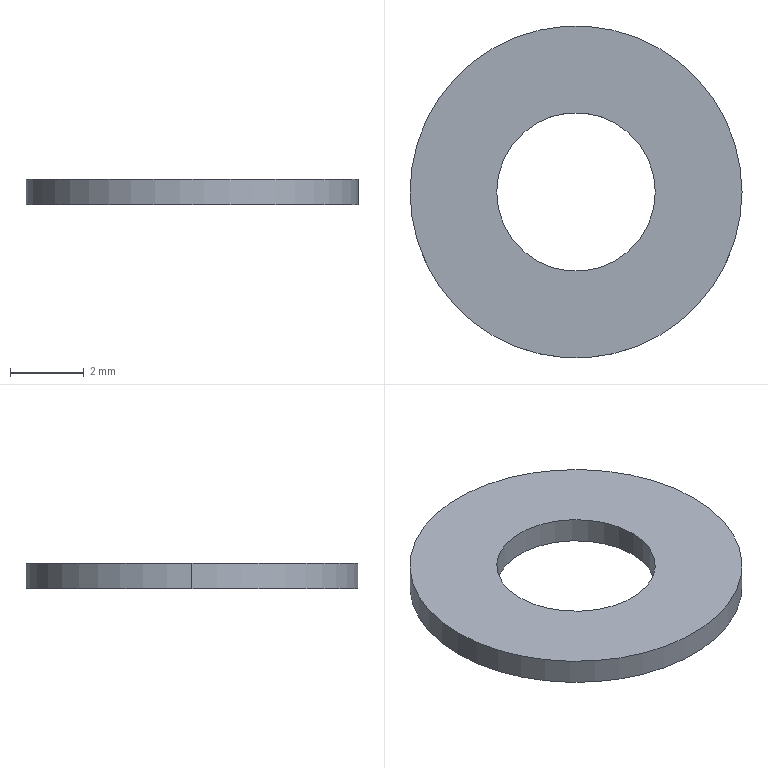Part | SolidWorks | features Extrusion 1, RefAxis 1 | 1 solid | 6 faces | box 9 x 9 x 0.7 mm | volume 34.367 mm3 | cylinder 4 | plane 2 | commonest cylinder face diameters 4.3 x2 9 x2
STEP:
#1=CARTESIAN_POINT('',(-2.15,0.,0.7));
#2=VERTEX_POINT('',#1);
#3=CARTESIAN_POINT('',(2.15,0.,0.7));
#4=VERTEX_POINT('',#3);
#5=CARTESIAN_POINT('',(0.,0.,0.7));
#6=DIRECTION('',(0.,0.,1.));
#7=DIRECTION('',(1.,0.,0.));
#8=AXIS2_PLACEMENT_3D('',#5,#6,#7);
#9=CIRCLE('',#8,2.15);
#10=EDGE_CURVE('',#2,#4,#9,.T.);
#11=ORIENTED_EDGE('',*,*,#10,.T.);
#12=CARTESIAN_POINT('',(2.15,0.,0.));
#13=VERTEX_POINT('',#12);
#14=CARTESIAN_POINT('',(2.15,0.,0.7));
#15=DIRECTION('',(0.,0.,-1.));
#16=VECTOR('',#15,1000.);
#17=LINE('',#14,#16);
#18=EDGE_CURVE('',#4,#13,#17,.T.);
#19=ORIENTED_EDGE('',*,*,#18,.T.);
#20=CARTESIAN_POINT('',(-2.15,0.,0.));
#21=VERTEX_POINT('',#20);
#22=CARTESIAN_POINT('',(0.,0.,0.));
#23=DIRECTION('',(0.,0.,1.));
#24=DIRECTION('',(1.,0.,0.));
#25=AXIS2_PLACEMENT_3D('',#22,#23,#24);
#26=CIRCLE('',#25,2.15);
#27=EDGE_CURVE('',#21,#13,#26,.T.);
#28=ORIENTED_EDGE('',*,*,#27,.F.);
#29=CARTESIAN_POINT('',(-2.15,0.,0.7));
#30=DIRECTION('',(0.,0.,-1.));
#31=VECTOR('',#30,1000.);
#32=LINE('',#29,#31);
#33=EDGE_CURVE('',#2,#21,#32,.T.);
#34=ORIENTED_EDGE('',*,*,#33,.F.);
#35=EDGE_LOOP('',(#11,#19,#28,#34));
#36=FACE_OUTER_BOUND('',#35,.T.);
#37=CARTESIAN_POINT('',(0.,0.,0.7));
#38=DIRECTION('',(0.,0.,-1.));
#39=DIRECTION('',(-1.,0.,0.));
#40=AXIS2_PLACEMENT_3D('',#37,#38,#39);
#41=CYLINDRICAL_SURFACE('',#40,2.15);
#42=ADVANCED_FACE('',(#36),#41,.F.);
#43=CARTESIAN_POINT('',(4.5,0.,0.7));
#44=VERTEX_POINT('',#43);
#45=CARTESIAN_POINT('',(-4.5,0.,0.7));
#46=VERTEX_POINT('',#45);
#47=CARTESIAN_POINT('',(0.,0.,0.7));
#48=DIRECTION('',(0.,0.,1.));
#49=DIRECTION('',(1.,0.,0.));
#50=AXIS2_PLACEMENT_3D('',#47,#48,#49);
#51=CIRCLE('',#50,4.5);
#52=EDGE_CURVE('',#44,#46,#51,.T.);
#53=ORIENTED_EDGE('',*,*,#52,.F.);
#54=CARTESIAN_POINT('',(4.5,0.,0.));
#55=VERTEX_POINT('',#54);
#56=CARTESIAN_POINT('',(4.5,0.,0.7));
#57=DIRECTION('',(0.,0.,-1.));
#58=VECTOR('',#57,1000.);
#59=LINE('',#56,#58);
#60=EDGE_CURVE('',#44,#55,#59,.T.);
#61=ORIENTED_EDGE('',*,*,#60,.T.);
#62=CARTESIAN_POINT('',(-4.5,0.,0.));
#63=VERTEX_POINT('',#62);
#64=CARTESIAN_POINT('',(0.,0.,0.));
#65=DIRECTION('',(0.,0.,1.));
#66=DIRECTION('',(1.,0.,0.));
#67=AXIS2_PLACEMENT_3D('',#64,#65,#66);
#68=CIRCLE('',#67,4.5);
#69=EDGE_CURVE('',#55,#63,#68,.T.);
#70=ORIENTED_EDGE('',*,*,#69,.T.);
#71=CARTESIAN_POINT('',(-4.5,0.,0.7));
#72=DIRECTION('',(0.,0.,-1.));
#73=VECTOR('',#72,1000.);
#74=LINE('',#71,#73);
#75=EDGE_CURVE('',#46,#63,#74,.T.);
#76=ORIENTED_EDGE('',*,*,#75,.F.);
#77=EDGE_LOOP('',(#53,#61,#70,#76));
#78=FACE_OUTER_BOUND('',#77,.T.);
#79=CARTESIAN_POINT('',(0.,0.,0.7));
#80=DIRECTION('',(0.,0.,-1.));
#81=DIRECTION('',(-1.,0.,0.));
#82=AXIS2_PLACEMENT_3D('',#79,#80,#81);
#83=CYLINDRICAL_SURFACE('',#82,4.5);
#84=ADVANCED_FACE('',(#78),#83,.T.);
#85=CARTESIAN_POINT('',(0.,0.,0.7));
#86=DIRECTION('',(0.,0.,1.));
#87=DIRECTION('',(1.,0.,0.));
#88=AXIS2_PLACEMENT_3D('',#85,#86,#87);
#89=CIRCLE('',#88,4.5);
#90=EDGE_CURVE('',#46,#44,#89,.T.);
#91=ORIENTED_EDGE('',*,*,#90,.T.);
#92=ORIENTED_EDGE('',*,*,#52,.T.);
#93=EDGE_LOOP('',(#91,#92));
#94=FACE_OUTER_BOUND('',#93,.T.);
#95=ORIENTED_EDGE('',*,*,#10,.F.);
#96=CARTESIAN_POINT('',(0.,0.,0.7));
#97=DIRECTION('',(0.,0.,1.));
#98=DIRECTION('',(1.,0.,0.));
#99=AXIS2_PLACEMENT_3D('',#96,#97,#98);
#100=CIRCLE('',#99,2.15);
#101=EDGE_CURVE('',#4,#2,#100,.T.);
#102=ORIENTED_EDGE('',*,*,#101,.F.);
#103=EDGE_LOOP('',(#95,#102));
#104=FACE_BOUND('',#103,.T.);
#105=CARTESIAN_POINT('',(0.,0.,0.7));
#106=DIRECTION('',(0.,0.,1.));
#107=DIRECTION('',(1.,0.,0.));
#108=AXIS2_PLACEMENT_3D('',#105,#106,#107);
#109=PLANE('',#108);
#110=ADVANCED_FACE('',(#94,#104),#109,.T.);
#111=CARTESIAN_POINT('',(0.,0.,0.));
#112=DIRECTION('',(0.,0.,1.));
#113=DIRECTION('',(1.,0.,0.));
#114=AXIS2_PLACEMENT_3D('',#111,#112,#113);
#115=CIRCLE('',#114,4.5);
#116=EDGE_CURVE('',#63,#55,#115,.T.);
#117=ORIENTED_EDGE('',*,*,#116,.F.);
#118=ORIENTED_EDGE('',*,*,#69,.F.);
#119=EDGE_LOOP('',(#117,#118));
#120=FACE_OUTER_BOUND('',#119,.T.);
#121=ORIENTED_EDGE('',*,*,#27,.T.);
#122=CARTESIAN_POINT('',(0.,0.,0.));
#123=DIRECTION('',(0.,0.,1.));
#124=DIRECTION('',(1.,0.,0.));
#125=AXIS2_PLACEMENT_3D('',#122,#123,#124);
#126=CIRCLE('',#125,2.15);
#127=EDGE_CURVE('',#13,#21,#126,.T.);
#128=ORIENTED_EDGE('',*,*,#127,.T.);
#129=EDGE_LOOP('',(#121,#128));
#130=FACE_BOUND('',#129,.T.);
#131=CARTESIAN_POINT('',(0.,0.,0.));
#132=DIRECTION('',(0.,0.,1.));
#133=DIRECTION('',(1.,0.,0.));
#134=AXIS2_PLACEMENT_3D('',#131,#132,#133);
#135=PLANE('',#134);
#136=ADVANCED_FACE('',(#120,#130),#135,.F.);
#137=ORIENTED_EDGE('',*,*,#60,.F.);
#138=ORIENTED_EDGE('',*,*,#90,.F.);
#139=ORIENTED_EDGE('',*,*,#75,.T.);
#140=ORIENTED_EDGE('',*,*,#116,.T.);
#141=EDGE_LOOP('',(#137,#138,#139,#140));
#142=FACE_OUTER_BOUND('',#141,.T.);
#143=CARTESIAN_POINT('',(0.,0.,0.7));
#144=DIRECTION('',(0.,0.,-1.));
#145=DIRECTION('',(-1.,0.,0.));
#146=AXIS2_PLACEMENT_3D('',#143,#144,#145);
#147=CYLINDRICAL_SURFACE('',#146,4.5);
#148=ADVANCED_FACE('',(#142),#147,.T.);
#149=ORIENTED_EDGE('',*,*,#18,.F.);
#150=ORIENTED_EDGE('',*,*,#101,.T.);
#151=ORIENTED_EDGE('',*,*,#33,.T.);
#152=ORIENTED_EDGE('',*,*,#127,.F.);
#153=EDGE_LOOP('',(#149,#150,#151,#152));
#154=FACE_OUTER_BOUND('',#153,.T.);
#155=CARTESIAN_POINT('',(0.,0.,0.7));
#156=DIRECTION('',(0.,0.,-1.));
#157=DIRECTION('',(-1.,0.,0.));
#158=AXIS2_PLACEMENT_3D('',#155,#156,#157);
#159=CYLINDRICAL_SURFACE('',#158,2.15);
#160=ADVANCED_FACE('',(#154),#159,.F.);
#161=CLOSED_SHELL('',(#42,#84,#110,#136,#148,#160));
#162=MANIFOLD_SOLID_BREP('',#161);
#163=CARTESIAN_POINT('',(0.,0.,0.));
#164=DIRECTION('',(0.,0.,1.));
#165=DIRECTION('',(1.,0.,0.));
#166=AXIS2_PLACEMENT_3D('',#163,#164,#165);
#167=(LENGTH_UNIT()NAMED_UNIT(*)SI_UNIT(.MILLI.,.METRE.));
#168=UNCERTAINTY_MEASURE_WITH_UNIT(LENGTH_MEASURE(0.00001),#167,'','');
#169=(NAMED_UNIT(*)PLANE_ANGLE_UNIT()SI_UNIT($,.RADIAN.));
#170=(NAMED_UNIT(*)SI_UNIT($,.STERADIAN.)SOLID_ANGLE_UNIT());
#171=(GEOMETRIC_REPRESENTATION_CONTEXT(3)GLOBAL_UNCERTAINTY_ASSIGNED_CONTEXT((#168))GLOBAL_UNIT_ASSIGNED_CONTEXT((#167,#169,#170))REPRESENTATION_CONTEXT('',''));
#172=ADVANCED_BREP_SHAPE_REPRESENTATION('',(#162,#166),#171);